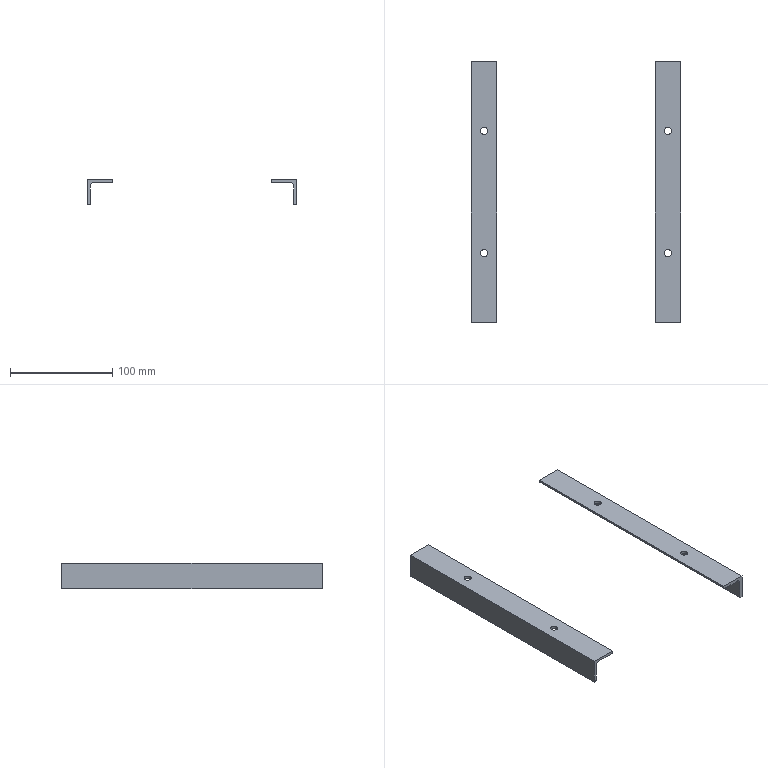Part | SolidWorks | features HoleWzd 1, WeldMemberFeat 1, WeldmentFeature 1 | 2 solids | 30 faces | box 205 x 255 x 25 mm | volume 72570 mm3 | plane 16 | cylinder 14 | commonest cylinder face diameters 7 x10 2 x4
STEP:
#1=CARTESIAN_POINT('',(-93.5,60.,-3.));
#2=VERTEX_POINT('',#1);
#3=CARTESIAN_POINT('',(-86.5,60.,-3.));
#4=VERTEX_POINT('',#3);
#5=CARTESIAN_POINT('',(-90.,60.,-3.));
#6=DIRECTION('',(0.,0.,1.));
#7=DIRECTION('',(1.,0.,0.));
#8=AXIS2_PLACEMENT_3D('',#5,#6,#7);
#9=CIRCLE('',#8,3.5);
#10=EDGE_CURVE('',#2,#4,#9,.T.);
#11=ORIENTED_EDGE('',*,*,#10,.F.);
#12=CARTESIAN_POINT('',(-93.5,60.,0.));
#13=VERTEX_POINT('',#12);
#14=CARTESIAN_POINT('',(-93.5,60.,0.));
#15=DIRECTION('',(0.,0.,1.));
#16=VECTOR('',#15,1000.);
#17=LINE('',#14,#16);
#18=EDGE_CURVE('',#2,#13,#17,.T.);
#19=ORIENTED_EDGE('',*,*,#18,.T.);
#20=CARTESIAN_POINT('',(-86.5,60.,0.));
#21=VERTEX_POINT('',#20);
#22=CARTESIAN_POINT('',(-90.,60.,0.));
#23=DIRECTION('',(0.,0.,1.));
#24=DIRECTION('',(1.,0.,0.));
#25=AXIS2_PLACEMENT_3D('',#22,#23,#24);
#26=CIRCLE('',#25,3.5);
#27=EDGE_CURVE('',#13,#21,#26,.T.);
#28=ORIENTED_EDGE('',*,*,#27,.T.);
#29=CARTESIAN_POINT('',(-86.5,60.,0.));
#30=DIRECTION('',(0.,0.,1.));
#31=VECTOR('',#30,1000.);
#32=LINE('',#29,#31);
#33=EDGE_CURVE('',#4,#21,#32,.T.);
#34=ORIENTED_EDGE('',*,*,#33,.F.);
#35=EDGE_LOOP('',(#11,#19,#28,#34));
#36=FACE_OUTER_BOUND('',#35,.T.);
#37=CARTESIAN_POINT('',(-90.,60.,0.));
#38=DIRECTION('',(0.,0.,1.));
#39=DIRECTION('',(1.,0.,0.));
#40=AXIS2_PLACEMENT_3D('',#37,#38,#39);
#41=CYLINDRICAL_SURFACE('',#40,3.5);
#42=ADVANCED_FACE('',(#36),#41,.F.);
#43=CARTESIAN_POINT('',(-93.5,-60.,-3.));
#44=VERTEX_POINT('',#43);
#45=CARTESIAN_POINT('',(-86.5,-60.,-3.));
#46=VERTEX_POINT('',#45);
#47=CARTESIAN_POINT('',(-90.,-60.,-3.));
#48=DIRECTION('',(0.,0.,1.));
#49=DIRECTION('',(1.,0.,0.));
#50=AXIS2_PLACEMENT_3D('',#47,#48,#49);
#51=CIRCLE('',#50,3.5);
#52=EDGE_CURVE('',#44,#46,#51,.T.);
#53=ORIENTED_EDGE('',*,*,#52,.F.);
#54=CARTESIAN_POINT('',(-93.5,-60.,0.));
#55=VERTEX_POINT('',#54);
#56=CARTESIAN_POINT('',(-93.5,-60.,0.));
#57=DIRECTION('',(0.,0.,1.));
#58=VECTOR('',#57,1000.);
#59=LINE('',#56,#58);
#60=EDGE_CURVE('',#44,#55,#59,.T.);
#61=ORIENTED_EDGE('',*,*,#60,.T.);
#62=CARTESIAN_POINT('',(-86.5,-60.,0.));
#63=VERTEX_POINT('',#62);
#64=CARTESIAN_POINT('',(-90.,-60.,0.));
#65=DIRECTION('',(0.,0.,1.));
#66=DIRECTION('',(1.,0.,0.));
#67=AXIS2_PLACEMENT_3D('',#64,#65,#66);
#68=CIRCLE('',#67,3.5);
#69=EDGE_CURVE('',#55,#63,#68,.T.);
#70=ORIENTED_EDGE('',*,*,#69,.T.);
#71=CARTESIAN_POINT('',(-86.5,-60.,0.));
#72=DIRECTION('',(0.,0.,1.));
#73=VECTOR('',#72,1000.);
#74=LINE('',#71,#73);
#75=EDGE_CURVE('',#46,#63,#74,.T.);
#76=ORIENTED_EDGE('',*,*,#75,.F.);
#77=EDGE_LOOP('',(#53,#61,#70,#76));
#78=FACE_OUTER_BOUND('',#77,.T.);
#79=CARTESIAN_POINT('',(-90.,-60.,0.));
#80=DIRECTION('',(0.,0.,1.));
#81=DIRECTION('',(1.,0.,0.));
#82=AXIS2_PLACEMENT_3D('',#79,#80,#81);
#83=CYLINDRICAL_SURFACE('',#82,3.5);
#84=ADVANCED_FACE('',(#78),#83,.F.);
#85=CARTESIAN_POINT('',(-100.5,-127.5,-25.));
#86=VERTEX_POINT('',#85);
#87=CARTESIAN_POINT('',(-102.5,-127.5,-25.));
#88=VERTEX_POINT('',#87);
#89=CARTESIAN_POINT('',(-102.5,-127.5,-25.));
#90=DIRECTION('',(-1.,0.,0.));
#91=VECTOR('',#90,1000.);
#92=LINE('',#89,#91);
#93=EDGE_CURVE('',#86,#88,#92,.T.);
#94=ORIENTED_EDGE('',*,*,#93,.T.);
#95=CARTESIAN_POINT('',(-102.5,127.5,-25.));
#96=VERTEX_POINT('',#95);
#97=CARTESIAN_POINT('',(-102.5,127.5,-25.));
#98=DIRECTION('',(0.,-1.,0.));
#99=VECTOR('',#98,1000.);
#100=LINE('',#97,#99);
#101=EDGE_CURVE('',#96,#88,#100,.T.);
#102=ORIENTED_EDGE('',*,*,#101,.F.);
#103=CARTESIAN_POINT('',(-100.5,127.5,-25.));
#104=VERTEX_POINT('',#103);
#105=CARTESIAN_POINT('',(-102.5,127.5,-25.));
#106=DIRECTION('',(-1.,0.,0.));
#107=VECTOR('',#106,1000.);
#108=LINE('',#105,#107);
#109=EDGE_CURVE('',#104,#96,#108,.T.);
#110=ORIENTED_EDGE('',*,*,#109,.F.);
#111=CARTESIAN_POINT('',(-100.5,127.5,-25.));
#112=DIRECTION('',(0.,-1.,0.));
#113=VECTOR('',#112,1000.);
#114=LINE('',#111,#113);
#115=EDGE_CURVE('',#104,#86,#114,.T.);
#116=ORIENTED_EDGE('',*,*,#115,.T.);
#117=EDGE_LOOP('',(#94,#102,#110,#116));
#118=FACE_OUTER_BOUND('',#117,.T.);
#119=CARTESIAN_POINT('',(-102.5,127.5,-25.));
#120=DIRECTION('',(0.,0.,1.));
#121=DIRECTION('',(1.,0.,0.));
#122=AXIS2_PLACEMENT_3D('',#119,#120,#121);
#123=PLANE('',#122);
#124=ADVANCED_FACE('',(#118),#123,.F.);
#125=CARTESIAN_POINT('',(-102.5,-127.5,0.));
#126=VERTEX_POINT('',#125);
#127=CARTESIAN_POINT('',(-102.5,-127.5,-25.));
#128=DIRECTION('',(0.,0.,1.));
#129=VECTOR('',#128,1000.);
#130=LINE('',#127,#129);
#131=EDGE_CURVE('',#88,#126,#130,.T.);
#132=ORIENTED_EDGE('',*,*,#131,.T.);
#133=CARTESIAN_POINT('',(-102.5,127.5,0.));
#134=VERTEX_POINT('',#133);
#135=CARTESIAN_POINT('',(-102.5,127.5,0.));
#136=DIRECTION('',(0.,-1.,0.));
#137=VECTOR('',#136,1000.);
#138=LINE('',#135,#137);
#139=EDGE_CURVE('',#134,#126,#138,.T.);
#140=ORIENTED_EDGE('',*,*,#139,.F.);
#141=CARTESIAN_POINT('',(-102.5,127.5,-25.));
#142=DIRECTION('',(0.,0.,1.));
#143=VECTOR('',#142,1000.);
#144=LINE('',#141,#143);
#145=EDGE_CURVE('',#96,#134,#144,.T.);
#146=ORIENTED_EDGE('',*,*,#145,.F.);
#147=ORIENTED_EDGE('',*,*,#101,.T.);
#148=EDGE_LOOP('',(#132,#140,#146,#147));
#149=FACE_OUTER_BOUND('',#148,.T.);
#150=CARTESIAN_POINT('',(-102.5,127.5,-25.));
#151=DIRECTION('',(1.,0.,0.));
#152=DIRECTION('',(0.,0.,-1.));
#153=AXIS2_PLACEMENT_3D('',#150,#151,#152);
#154=PLANE('',#153);
#155=ADVANCED_FACE('',(#149),#154,.F.);
#156=CARTESIAN_POINT('',(-90.,60.,0.));
#157=DIRECTION('',(0.,0.,1.));
#158=DIRECTION('',(1.,0.,0.));
#159=AXIS2_PLACEMENT_3D('',#156,#157,#158);
#160=CIRCLE('',#159,3.5);
#161=EDGE_CURVE('',#21,#13,#160,.T.);
#162=ORIENTED_EDGE('',*,*,#161,.F.);
#163=ORIENTED_EDGE('',*,*,#27,.F.);
#164=EDGE_LOOP('',(#162,#163));
#165=FACE_BOUND('',#164,.T.);
#166=CARTESIAN_POINT('',(-90.,-60.,0.));
#167=DIRECTION('',(0.,0.,1.));
#168=DIRECTION('',(1.,0.,0.));
#169=AXIS2_PLACEMENT_3D('',#166,#167,#168);
#170=CIRCLE('',#169,3.5);
#171=EDGE_CURVE('',#63,#55,#170,.T.);
#172=ORIENTED_EDGE('',*,*,#171,.F.);
#173=ORIENTED_EDGE('',*,*,#69,.F.);
#174=EDGE_LOOP('',(#172,#173));
#175=FACE_BOUND('',#174,.T.);
#176=CARTESIAN_POINT('',(-77.5,-127.5,0.));
#177=VERTEX_POINT('',#176);
#178=CARTESIAN_POINT('',(-102.5,-127.5,0.));
#179=DIRECTION('',(1.,0.,0.));
#180=VECTOR('',#179,1000.);
#181=LINE('',#178,#180);
#182=EDGE_CURVE('',#126,#177,#181,.T.);
#183=ORIENTED_EDGE('',*,*,#182,.T.);
#184=CARTESIAN_POINT('',(-77.5,127.5,0.));
#185=VERTEX_POINT('',#184);
#186=CARTESIAN_POINT('',(-77.5,127.5,0.));
#187=DIRECTION('',(0.,-1.,0.));
#188=VECTOR('',#187,1000.);
#189=LINE('',#186,#188);
#190=EDGE_CURVE('',#185,#177,#189,.T.);
#191=ORIENTED_EDGE('',*,*,#190,.F.);
#192=CARTESIAN_POINT('',(-102.5,127.5,0.));
#193=DIRECTION('',(1.,0.,0.));
#194=VECTOR('',#193,1000.);
#195=LINE('',#192,#194);
#196=EDGE_CURVE('',#134,#185,#195,.T.);
#197=ORIENTED_EDGE('',*,*,#196,.F.);
#198=ORIENTED_EDGE('',*,*,#139,.T.);
#199=EDGE_LOOP('',(#183,#191,#197,#198));
#200=FACE_OUTER_BOUND('',#199,.T.);
#201=CARTESIAN_POINT('',(-102.5,127.5,0.));
#202=DIRECTION('',(0.,0.,-1.));
#203=DIRECTION('',(-1.,0.,0.));
#204=AXIS2_PLACEMENT_3D('',#201,#202,#203);
#205=PLANE('',#204);
#206=ADVANCED_FACE('',(#165,#175,#200),#205,.F.);
#207=CARTESIAN_POINT('',(-77.5,-127.5,-2.));
#208=VERTEX_POINT('',#207);
#209=CARTESIAN_POINT('',(-77.5,-127.5,0.));
#210=DIRECTION('',(0.,0.,-1.));
#211=VECTOR('',#210,1000.);
#212=LINE('',#209,#211);
#213=EDGE_CURVE('',#177,#208,#212,.T.);
#214=ORIENTED_EDGE('',*,*,#213,.T.);
#215=CARTESIAN_POINT('',(-77.5,127.5,-2.));
#216=VERTEX_POINT('',#215);
#217=CARTESIAN_POINT('',(-77.5,127.5,-2.));
#218=DIRECTION('',(0.,-1.,0.));
#219=VECTOR('',#218,1000.);
#220=LINE('',#217,#219);
#221=EDGE_CURVE('',#216,#208,#220,.T.);
#222=ORIENTED_EDGE('',*,*,#221,.F.);
#223=CARTESIAN_POINT('',(-77.5,127.5,0.));
#224=DIRECTION('',(0.,0.,-1.));
#225=VECTOR('',#224,1000.);
#226=LINE('',#223,#225);
#227=EDGE_CURVE('',#185,#216,#226,.T.);
#228=ORIENTED_EDGE('',*,*,#227,.F.);
#229=ORIENTED_EDGE('',*,*,#190,.T.);
#230=EDGE_LOOP('',(#214,#222,#228,#229));
#231=FACE_OUTER_BOUND('',#230,.T.);
#232=CARTESIAN_POINT('',(-77.5,127.5,0.));
#233=DIRECTION('',(-1.,0.,0.));
#234=DIRECTION('',(0.,0.,1.));
#235=AXIS2_PLACEMENT_3D('',#232,#233,#234);
#236=PLANE('',#235);
#237=ADVANCED_FACE('',(#231),#236,.F.);
#238=CARTESIAN_POINT('',(-78.5,-127.5,-3.));
#239=VERTEX_POINT('',#238);
#240=CARTESIAN_POINT('',(-78.5,-127.5,-2.));
#241=DIRECTION('',(0.,1.,0.));
#242=DIRECTION('',(0.,0.,1.));
#243=AXIS2_PLACEMENT_3D('',#240,#241,#242);
#244=CIRCLE('',#243,1.);
#245=EDGE_CURVE('',#208,#239,#244,.T.);
#246=ORIENTED_EDGE('',*,*,#245,.T.);
#247=CARTESIAN_POINT('',(-78.5,127.5,-3.));
#248=VERTEX_POINT('',#247);
#249=CARTESIAN_POINT('',(-78.5,127.5,-3.));
#250=DIRECTION('',(0.,-1.,0.));
#251=VECTOR('',#250,1000.);
#252=LINE('',#249,#251);
#253=EDGE_CURVE('',#248,#239,#252,.T.);
#254=ORIENTED_EDGE('',*,*,#253,.F.);
#255=CARTESIAN_POINT('',(-78.5,127.5,-2.));
#256=DIRECTION('',(0.,1.,0.));
#257=DIRECTION('',(0.,0.,1.));
#258=AXIS2_PLACEMENT_3D('',#255,#256,#257);
#259=CIRCLE('',#258,1.);
#260=EDGE_CURVE('',#216,#248,#259,.T.);
#261=ORIENTED_EDGE('',*,*,#260,.F.);
#262=ORIENTED_EDGE('',*,*,#221,.T.);
#263=EDGE_LOOP('',(#246,#254,#261,#262));
#264=FACE_OUTER_BOUND('',#263,.T.);
#265=CARTESIAN_POINT('',(-78.5,127.5,-2.));
#266=DIRECTION('',(0.,-1.,0.));
#267=DIRECTION('',(0.,0.,-1.));
#268=AXIS2_PLACEMENT_3D('',#265,#266,#267);
#269=CYLINDRICAL_SURFACE('',#268,1.);
#270=ADVANCED_FACE('',(#264),#269,.T.);
#271=CARTESIAN_POINT('',(-90.,60.,-3.));
#272=DIRECTION('',(0.,0.,1.));
#273=DIRECTION('',(1.,0.,0.));
#274=AXIS2_PLACEMENT_3D('',#271,#272,#273);
#275=CIRCLE('',#274,3.5);
#276=EDGE_CURVE('',#4,#2,#275,.T.);
#277=ORIENTED_EDGE('',*,*,#276,.T.);
#278=ORIENTED_EDGE('',*,*,#10,.T.);
#279=EDGE_LOOP('',(#277,#278));
#280=FACE_BOUND('',#279,.T.);
#281=CARTESIAN_POINT('',(-90.,-60.,-3.));
#282=DIRECTION('',(0.,0.,1.));
#283=DIRECTION('',(1.,0.,0.));
#284=AXIS2_PLACEMENT_3D('',#281,#282,#283);
#285=CIRCLE('',#284,3.5);
#286=EDGE_CURVE('',#46,#44,#285,.T.);
#287=ORIENTED_EDGE('',*,*,#286,.T.);
#288=ORIENTED_EDGE('',*,*,#52,.T.);
#289=EDGE_LOOP('',(#287,#288));
#290=FACE_BOUND('',#289,.T.);
#291=CARTESIAN_POINT('',(-96.,-127.5,-3.));
#292=VERTEX_POINT('',#291);
#293=CARTESIAN_POINT('',(-96.,-127.5,-3.));
#294=DIRECTION('',(-1.,0.,0.));
#295=VECTOR('',#294,1000.);
#296=LINE('',#293,#295);
#297=EDGE_CURVE('',#239,#292,#296,.T.);
#298=ORIENTED_EDGE('',*,*,#297,.T.);
#299=CARTESIAN_POINT('',(-96.,127.5,-3.));
#300=VERTEX_POINT('',#299);
#301=CARTESIAN_POINT('',(-96.,127.5,-3.));
#302=DIRECTION('',(0.,-1.,0.));
#303=VECTOR('',#302,1000.);
#304=LINE('',#301,#303);
#305=EDGE_CURVE('',#300,#292,#304,.T.);
#306=ORIENTED_EDGE('',*,*,#305,.F.);
#307=CARTESIAN_POINT('',(-96.,127.5,-3.));
#308=DIRECTION('',(-1.,0.,0.));
#309=VECTOR('',#308,1000.);
#310=LINE('',#307,#309);
#311=EDGE_CURVE('',#248,#300,#310,.T.);
#312=ORIENTED_EDGE('',*,*,#311,.F.);
#313=ORIENTED_EDGE('',*,*,#253,.T.);
#314=EDGE_LOOP('',(#298,#306,#312,#313));
#315=FACE_OUTER_BOUND('',#314,.T.);
#316=CARTESIAN_POINT('',(-96.,127.5,-3.));
#317=DIRECTION('',(0.,0.,1.));
#318=DIRECTION('',(1.,0.,0.));
#319=AXIS2_PLACEMENT_3D('',#316,#317,#318);
#320=PLANE('',#319);
#321=ADVANCED_FACE('',(#280,#290,#315),#320,.F.);
#322=CARTESIAN_POINT('',(-99.5,-127.5,-6.5));
#323=VERTEX_POINT('',#322);
#324=CARTESIAN_POINT('',(-96.,-127.5,-6.5));
#325=DIRECTION('',(0.,-1.,0.));
#326=DIRECTION('',(0.,0.,1.));
#327=AXIS2_PLACEMENT_3D('',#324,#325,#326);
#328=CIRCLE('',#327,3.5);
#329=EDGE_CURVE('',#292,#323,#328,.T.);
#330=ORIENTED_EDGE('',*,*,#329,.T.);
#331=CARTESIAN_POINT('',(-99.5,127.5,-6.5));
#332=VERTEX_POINT('',#331);
#333=CARTESIAN_POINT('',(-99.5,127.5,-6.5));
#334=DIRECTION('',(0.,-1.,0.));
#335=VECTOR('',#334,1000.);
#336=LINE('',#333,#335);
#337=EDGE_CURVE('',#332,#323,#336,.T.);
#338=ORIENTED_EDGE('',*,*,#337,.F.);
#339=CARTESIAN_POINT('',(-96.,127.5,-6.5));
#340=DIRECTION('',(0.,-1.,0.));
#341=DIRECTION('',(0.,0.,1.));
#342=AXIS2_PLACEMENT_3D('',#339,#340,#341);
#343=CIRCLE('',#342,3.5);
#344=EDGE_CURVE('',#300,#332,#343,.T.);
#345=ORIENTED_EDGE('',*,*,#344,.F.);
#346=ORIENTED_EDGE('',*,*,#305,.T.);
#347=EDGE_LOOP('',(#330,#338,#345,#346));
#348=FACE_OUTER_BOUND('',#347,.T.);
#349=CARTESIAN_POINT('',(-96.,127.5,-6.5));
#350=DIRECTION('',(0.,-1.,0.));
#351=DIRECTION('',(0.,0.,-1.));
#352=AXIS2_PLACEMENT_3D('',#349,#350,#351);
#353=CYLINDRICAL_SURFACE('',#352,3.5);
#354=ADVANCED_FACE('',(#348),#353,.F.);
#355=CARTESIAN_POINT('',(-99.5,-127.5,-24.));
#356=VERTEX_POINT('',#355);
#357=CARTESIAN_POINT('',(-99.5,-127.5,-24.));
#358=DIRECTION('',(0.,0.,-1.));
#359=VECTOR('',#358,1000.);
#360=LINE('',#357,#359);
#361=EDGE_CURVE('',#323,#356,#360,.T.);
#362=ORIENTED_EDGE('',*,*,#361,.T.);
#363=CARTESIAN_POINT('',(-99.5,127.5,-24.));
#364=VERTEX_POINT('',#363);
#365=CARTESIAN_POINT('',(-99.5,127.5,-24.));
#366=DIRECTION('',(0.,-1.,0.));
#367=VECTOR('',#366,1000.);
#368=LINE('',#365,#367);
#369=EDGE_CURVE('',#364,#356,#368,.T.);
#370=ORIENTED_EDGE('',*,*,#369,.F.);
#371=CARTESIAN_POINT('',(-99.5,127.5,-24.));
#372=DIRECTION('',(0.,0.,-1.));
#373=VECTOR('',#372,1000.);
#374=LINE('',#371,#373);
#375=EDGE_CURVE('',#332,#364,#374,.T.);
#376=ORIENTED_EDGE('',*,*,#375,.F.);
#377=ORIENTED_EDGE('',*,*,#337,.T.);
#378=EDGE_LOOP('',(#362,#370,#376,#377));
#379=FACE_OUTER_BOUND('',#378,.T.);
#380=CARTESIAN_POINT('',(-99.5,127.5,-24.));
#381=DIRECTION('',(-1.,0.,0.));
#382=DIRECTION('',(0.,0.,1.));
#383=AXIS2_PLACEMENT_3D('',#380,#381,#382);
#384=PLANE('',#383);
#385=ADVANCED_FACE('',(#379),#384,.F.);
#386=CARTESIAN_POINT('',(-100.5,-127.5,-24.));
#387=DIRECTION('',(0.,1.,0.));
#388=DIRECTION('',(0.,0.,-1.));
#389=AXIS2_PLACEMENT_3D('',#386,#387,#388);
#390=CIRCLE('',#389,1.);
#391=EDGE_CURVE('',#356,#86,#390,.T.);
#392=ORIENTED_EDGE('',*,*,#391,.T.);
#393=ORIENTED_EDGE('',*,*,#115,.F.);
#394=CARTESIAN_POINT('',(-100.5,127.5,-24.));
#395=DIRECTION('',(0.,1.,0.));
#396=DIRECTION('',(0.,0.,-1.));
#397=AXIS2_PLACEMENT_3D('',#394,#395,#396);
#398=CIRCLE('',#397,1.);
#399=EDGE_CURVE('',#364,#104,#398,.T.);
#400=ORIENTED_EDGE('',*,*,#399,.F.);
#401=ORIENTED_EDGE('',*,*,#369,.T.);
#402=EDGE_LOOP('',(#392,#393,#400,#401));
#403=FACE_OUTER_BOUND('',#402,.T.);
#404=CARTESIAN_POINT('',(-100.5,127.5,-24.));
#405=DIRECTION('',(0.,-1.,0.));
#406=DIRECTION('',(0.,0.,-1.));
#407=AXIS2_PLACEMENT_3D('',#404,#405,#406);
#408=CYLINDRICAL_SURFACE('',#407,1.);
#409=ADVANCED_FACE('',(#403),#408,.T.);
#410=ORIENTED_EDGE('',*,*,#109,.T.);
#411=ORIENTED_EDGE('',*,*,#145,.T.);
#412=ORIENTED_EDGE('',*,*,#196,.T.);
#413=ORIENTED_EDGE('',*,*,#227,.T.);
#414=ORIENTED_EDGE('',*,*,#260,.T.);
#415=ORIENTED_EDGE('',*,*,#311,.T.);
#416=ORIENTED_EDGE('',*,*,#344,.T.);
#417=ORIENTED_EDGE('',*,*,#375,.T.);
#418=ORIENTED_EDGE('',*,*,#399,.T.);
#419=EDGE_LOOP('',(#410,#411,#412,#413,#414,#415,#416,#417,#418));
#420=FACE_OUTER_BOUND('',#419,.T.);
#421=CARTESIAN_POINT('',(-100.5,127.5,-24.));
#422=DIRECTION('',(0.,-1.,0.));
#423=DIRECTION('',(0.,0.,-1.));
#424=AXIS2_PLACEMENT_3D('',#421,#422,#423);
#425=PLANE('',#424);
#426=ADVANCED_FACE('',(#420),#425,.F.);
#427=ORIENTED_EDGE('',*,*,#93,.F.);
#428=ORIENTED_EDGE('',*,*,#391,.F.);
#429=ORIENTED_EDGE('',*,*,#361,.F.);
#430=ORIENTED_EDGE('',*,*,#329,.F.);
#431=ORIENTED_EDGE('',*,*,#297,.F.);
#432=ORIENTED_EDGE('',*,*,#245,.F.);
#433=ORIENTED_EDGE('',*,*,#213,.F.);
#434=ORIENTED_EDGE('',*,*,#182,.F.);
#435=ORIENTED_EDGE('',*,*,#131,.F.);
#436=EDGE_LOOP('',(#427,#428,#429,#430,#431,#432,#433,#434,#435));
#437=FACE_OUTER_BOUND('',#436,.T.);
#438=CARTESIAN_POINT('',(-100.5,-127.5,-24.));
#439=DIRECTION('',(0.,-1.,0.));
#440=DIRECTION('',(0.,0.,-1.));
#441=AXIS2_PLACEMENT_3D('',#438,#439,#440);
#442=PLANE('',#441);
#443=ADVANCED_FACE('',(#437),#442,.T.);
#444=ORIENTED_EDGE('',*,*,#60,.F.);
#445=ORIENTED_EDGE('',*,*,#286,.F.);
#446=ORIENTED_EDGE('',*,*,#75,.T.);
#447=ORIENTED_EDGE('',*,*,#171,.T.);
#448=EDGE_LOOP('',(#444,#445,#446,#447));
#449=FACE_OUTER_BOUND('',#448,.T.);
#450=CARTESIAN_POINT('',(-90.,-60.,0.));
#451=DIRECTION('',(0.,0.,1.));
#452=DIRECTION('',(1.,0.,0.));
#453=AXIS2_PLACEMENT_3D('',#450,#451,#452);
#454=CYLINDRICAL_SURFACE('',#453,3.5);
#455=ADVANCED_FACE('',(#449),#454,.F.);
#456=ORIENTED_EDGE('',*,*,#18,.F.);
#457=ORIENTED_EDGE('',*,*,#276,.F.);
#458=ORIENTED_EDGE('',*,*,#33,.T.);
#459=ORIENTED_EDGE('',*,*,#161,.T.);
#460=EDGE_LOOP('',(#456,#457,#458,#459));
#461=FACE_OUTER_BOUND('',#460,.T.);
#462=CARTESIAN_POINT('',(-90.,60.,0.));
#463=DIRECTION('',(0.,0.,1.));
#464=DIRECTION('',(1.,0.,0.));
#465=AXIS2_PLACEMENT_3D('',#462,#463,#464);
#466=CYLINDRICAL_SURFACE('',#465,3.5);
#467=ADVANCED_FACE('',(#461),#466,.F.);
#468=CLOSED_SHELL('',(#42,#84,#124,#155,#206,#237,#270,#321,#354,#385,#409,#426,#443,#455,#467));
#469=MANIFOLD_SOLID_BREP('',#468);
#470=CARTESIAN_POINT('',(93.5,-60.,-3.));
#471=VERTEX_POINT('',#470);
#472=CARTESIAN_POINT('',(86.5,-60.,-3.));
#473=VERTEX_POINT('',#472);
#474=CARTESIAN_POINT('',(90.,-60.,-3.));
#475=DIRECTION('',(0.,0.,-1.));
#476=DIRECTION('',(-1.,0.,0.));
#477=AXIS2_PLACEMENT_3D('',#474,#475,#476);
#478=CIRCLE('',#477,3.5);
#479=EDGE_CURVE('',#471,#473,#478,.T.);
#480=ORIENTED_EDGE('',*,*,#479,.T.);
#481=CARTESIAN_POINT('',(86.5,-60.,0.));
#482=VERTEX_POINT('',#481);
#483=CARTESIAN_POINT('',(86.5,-60.,0.));
#484=DIRECTION('',(0.,0.,1.));
#485=VECTOR('',#484,1000.);
#486=LINE('',#483,#485);
#487=EDGE_CURVE('',#473,#482,#486,.T.);
#488=ORIENTED_EDGE('',*,*,#487,.T.);
#489=CARTESIAN_POINT('',(93.5,-60.,0.));
#490=VERTEX_POINT('',#489);
#491=CARTESIAN_POINT('',(90.,-60.,0.));
#492=DIRECTION('',(0.,0.,1.));
#493=DIRECTION('',(1.,0.,0.));
#494=AXIS2_PLACEMENT_3D('',#491,#492,#493);
#495=CIRCLE('',#494,3.5);
#496=EDGE_CURVE('',#482,#490,#495,.T.);
#497=ORIENTED_EDGE('',*,*,#496,.T.);
#498=CARTESIAN_POINT('',(93.5,-60.,0.));
#499=DIRECTION('',(0.,0.,1.));
#500=VECTOR('',#499,1000.);
#501=LINE('',#498,#500);
#502=EDGE_CURVE('',#471,#490,#501,.T.);
#503=ORIENTED_EDGE('',*,*,#502,.F.);
#504=EDGE_LOOP('',(#480,#488,#497,#503));
#505=FACE_OUTER_BOUND('',#504,.T.);
#506=CARTESIAN_POINT('',(90.,-60.,0.));
#507=DIRECTION('',(0.,0.,1.));
#508=DIRECTION('',(1.,0.,0.));
#509=AXIS2_PLACEMENT_3D('',#506,#507,#508);
#510=CYLINDRICAL_SURFACE('',#509,3.5);
#511=ADVANCED_FACE('',(#505),#510,.F.);
#512=CARTESIAN_POINT('',(93.5,60.,-3.));
#513=VERTEX_POINT('',#512);
#514=CARTESIAN_POINT('',(86.5,60.,-3.));
#515=VERTEX_POINT('',#514);
#516=CARTESIAN_POINT('',(90.,60.,-3.));
#517=DIRECTION('',(0.,0.,-1.));
#518=DIRECTION('',(-1.,0.,0.));
#519=AXIS2_PLACEMENT_3D('',#516,#517,#518);
#520=CIRCLE('',#519,3.5);
#521=EDGE_CURVE('',#513,#515,#520,.T.);
#522=ORIENTED_EDGE('',*,*,#521,.T.);
#523=CARTESIAN_POINT('',(86.5,60.,0.));
#524=VERTEX_POINT('',#523);
#525=CARTESIAN_POINT('',(86.5,60.,0.));
#526=DIRECTION('',(0.,0.,1.));
#527=VECTOR('',#526,1000.);
#528=LINE('',#525,#527);
#529=EDGE_CURVE('',#515,#524,#528,.T.);
#530=ORIENTED_EDGE('',*,*,#529,.T.);
#531=CARTESIAN_POINT('',(93.5,60.,0.));
#532=VERTEX_POINT('',#531);
#533=CARTESIAN_POINT('',(90.,60.,0.));
#534=DIRECTION('',(0.,0.,1.));
#535=DIRECTION('',(1.,0.,0.));
#536=AXIS2_PLACEMENT_3D('',#533,#534,#535);
#537=CIRCLE('',#536,3.5);
#538=EDGE_CURVE('',#524,#532,#537,.T.);
#539=ORIENTED_EDGE('',*,*,#538,.T.);
#540=CARTESIAN_POINT('',(93.5,60.,0.));
#541=DIRECTION('',(0.,0.,1.));
#542=VECTOR('',#541,1000.);
#543=LINE('',#540,#542);
#544=EDGE_CURVE('',#513,#532,#543,.T.);
#545=ORIENTED_EDGE('',*,*,#544,.F.);
#546=EDGE_LOOP('',(#522,#530,#539,#545));
#547=FACE_OUTER_BOUND('',#546,.T.);
#548=CARTESIAN_POINT('',(90.,60.,0.));
#549=DIRECTION('',(0.,0.,1.));
#550=DIRECTION('',(1.,0.,0.));
#551=AXIS2_PLACEMENT_3D('',#548,#549,#550);
#552=CYLINDRICAL_SURFACE('',#551,3.5);
#553=ADVANCED_FACE('',(#547),#552,.F.);
#554=CARTESIAN_POINT('',(77.5,127.5,-2.));
#555=VERTEX_POINT('',#554);
#556=CARTESIAN_POINT('',(77.5,127.5,0.));
#557=VERTEX_POINT('',#556);
#558=CARTESIAN_POINT('',(77.5,127.5,0.));
#559=DIRECTION('',(0.,0.,1.));
#560=VECTOR('',#559,1000.);
#561=LINE('',#558,#560);
#562=EDGE_CURVE('',#555,#557,#561,.T.);
#563=ORIENTED_EDGE('',*,*,#562,.F.);
#564=CARTESIAN_POINT('',(77.5,-127.5,-2.));
#565=VERTEX_POINT('',#564);
#566=CARTESIAN_POINT('',(77.5,-127.5,-2.));
#567=DIRECTION('',(0.,1.,0.));
#568=VECTOR('',#567,1000.);
#569=LINE('',#566,#568);
#570=EDGE_CURVE('',#565,#555,#569,.T.);
#571=ORIENTED_EDGE('',*,*,#570,.F.);
#572=CARTESIAN_POINT('',(77.5,-127.5,0.));
#573=VERTEX_POINT('',#572);
#574=CARTESIAN_POINT('',(77.5,-127.5,0.));
#575=DIRECTION('',(0.,0.,1.));
#576=VECTOR('',#575,1000.);
#577=LINE('',#574,#576);
#578=EDGE_CURVE('',#565,#573,#577,.T.);
#579=ORIENTED_EDGE('',*,*,#578,.T.);
#580=CARTESIAN_POINT('',(77.5,-127.5,0.));
#581=DIRECTION('',(0.,1.,0.));
#582=VECTOR('',#581,1000.);
#583=LINE('',#580,#582);
#584=EDGE_CURVE('',#573,#557,#583,.T.);
#585=ORIENTED_EDGE('',*,*,#584,.T.);
#586=EDGE_LOOP('',(#563,#571,#579,#585));
#587=FACE_OUTER_BOUND('',#586,.T.);
#588=CARTESIAN_POINT('',(77.5,-127.5,0.));
#589=DIRECTION('',(-1.,0.,0.));
#590=DIRECTION('',(0.,0.,1.));
#591=AXIS2_PLACEMENT_3D('',#588,#589,#590);
#592=PLANE('',#591);
#593=ADVANCED_FACE('',(#587),#592,.T.);
#594=CARTESIAN_POINT('',(78.5,127.5,-3.));
#595=VERTEX_POINT('',#594);
#596=CARTESIAN_POINT('',(78.5,127.5,-2.));
#597=DIRECTION('',(0.,1.,0.));
#598=DIRECTION('',(-1.,0.,0.));
#599=AXIS2_PLACEMENT_3D('',#596,#597,#598);
#600=CIRCLE('',#599,1.);
#601=EDGE_CURVE('',#595,#555,#600,.T.);
#602=ORIENTED_EDGE('',*,*,#601,.F.);
#603=CARTESIAN_POINT('',(78.5,-127.5,-3.));
#604=VERTEX_POINT('',#603);
#605=CARTESIAN_POINT('',(78.5,-127.5,-3.));
#606=DIRECTION('',(0.,1.,0.));
#607=VECTOR('',#606,1000.);
#608=LINE('',#605,#607);
#609=EDGE_CURVE('',#604,#595,#608,.T.);
#610=ORIENTED_EDGE('',*,*,#609,.F.);
#611=CARTESIAN_POINT('',(78.5,-127.5,-2.));
#612=DIRECTION('',(0.,1.,0.));
#613=DIRECTION('',(-1.,0.,0.));
#614=AXIS2_PLACEMENT_3D('',#611,#612,#613);
#615=CIRCLE('',#614,1.);
#616=EDGE_CURVE('',#604,#565,#615,.T.);
#617=ORIENTED_EDGE('',*,*,#616,.T.);
#618=ORIENTED_EDGE('',*,*,#570,.T.);
#619=EDGE_LOOP('',(#602,#610,#617,#618));
#620=FACE_OUTER_BOUND('',#619,.T.);
#621=CARTESIAN_POINT('',(78.5,-127.5,-2.));
#622=DIRECTION('',(0.,1.,0.));
#623=DIRECTION('',(0.,0.,1.));
#624=AXIS2_PLACEMENT_3D('',#621,#622,#623);
#625=CYLINDRICAL_SURFACE('',#624,1.);
#626=ADVANCED_FACE('',(#620),#625,.T.);
#627=ORIENTED_EDGE('',*,*,#479,.F.);
#628=CARTESIAN_POINT('',(90.,-60.,-3.));
#629=DIRECTION('',(0.,0.,-1.));
#630=DIRECTION('',(-1.,0.,0.));
#631=AXIS2_PLACEMENT_3D('',#628,#629,#630);
#632=CIRCLE('',#631,3.5);
#633=EDGE_CURVE('',#473,#471,#632,.T.);
#634=ORIENTED_EDGE('',*,*,#633,.F.);
#635=EDGE_LOOP('',(#627,#634));
#636=FACE_BOUND('',#635,.T.);
#637=ORIENTED_EDGE('',*,*,#521,.F.);
#638=CARTESIAN_POINT('',(90.,60.,-3.));
#639=DIRECTION('',(0.,0.,-1.));
#640=DIRECTION('',(-1.,0.,0.));
#641=AXIS2_PLACEMENT_3D('',#638,#639,#640);
#642=CIRCLE('',#641,3.5);
#643=EDGE_CURVE('',#515,#513,#642,.T.);
#644=ORIENTED_EDGE('',*,*,#643,.F.);
#645=EDGE_LOOP('',(#637,#644));
#646=FACE_BOUND('',#645,.T.);
#647=CARTESIAN_POINT('',(96.,127.5,-3.));
#648=VERTEX_POINT('',#647);
#649=CARTESIAN_POINT('',(78.5,127.5,-3.));
#650=DIRECTION('',(-1.,0.,0.));
#651=VECTOR('',#650,1000.);
#652=LINE('',#649,#651);
#653=EDGE_CURVE('',#648,#595,#652,.T.);
#654=ORIENTED_EDGE('',*,*,#653,.F.);
#655=CARTESIAN_POINT('',(96.,-127.5,-3.));
#656=VERTEX_POINT('',#655);
#657=CARTESIAN_POINT('',(96.,-127.5,-3.));
#658=DIRECTION('',(0.,1.,0.));
#659=VECTOR('',#658,1000.);
#660=LINE('',#657,#659);
#661=EDGE_CURVE('',#656,#648,#660,.T.);
#662=ORIENTED_EDGE('',*,*,#661,.F.);
#663=CARTESIAN_POINT('',(78.5,-127.5,-3.));
#664=DIRECTION('',(-1.,0.,0.));
#665=VECTOR('',#664,1000.);
#666=LINE('',#663,#665);
#667=EDGE_CURVE('',#656,#604,#666,.T.);
#668=ORIENTED_EDGE('',*,*,#667,.T.);
#669=ORIENTED_EDGE('',*,*,#609,.T.);
#670=EDGE_LOOP('',(#654,#662,#668,#669));
#671=FACE_OUTER_BOUND('',#670,.T.);
#672=CARTESIAN_POINT('',(78.5,-127.5,-3.));
#673=DIRECTION('',(0.,0.,-1.));
#674=DIRECTION('',(-1.,0.,0.));
#675=AXIS2_PLACEMENT_3D('',#672,#673,#674);
#676=PLANE('',#675);
#677=ADVANCED_FACE('',(#636,#646,#671),#676,.T.);
#678=CARTESIAN_POINT('',(99.5,127.5,-6.5));
#679=VERTEX_POINT('',#678);
#680=CARTESIAN_POINT('',(96.,127.5,-6.5));
#681=DIRECTION('',(0.,-1.,0.));
#682=DIRECTION('',(1.,0.,0.));
#683=AXIS2_PLACEMENT_3D('',#680,#681,#682);
#684=CIRCLE('',#683,3.5);
#685=EDGE_CURVE('',#679,#648,#684,.T.);
#686=ORIENTED_EDGE('',*,*,#685,.F.);
#687=CARTESIAN_POINT('',(99.5,-127.5,-6.5));
#688=VERTEX_POINT('',#687);
#689=CARTESIAN_POINT('',(99.5,-127.5,-6.5));
#690=DIRECTION('',(0.,1.,0.));
#691=VECTOR('',#690,1000.);
#692=LINE('',#689,#691);
#693=EDGE_CURVE('',#688,#679,#692,.T.);
#694=ORIENTED_EDGE('',*,*,#693,.F.);
#695=CARTESIAN_POINT('',(96.,-127.5,-6.5));
#696=DIRECTION('',(0.,-1.,0.));
#697=DIRECTION('',(1.,0.,0.));
#698=AXIS2_PLACEMENT_3D('',#695,#696,#697);
#699=CIRCLE('',#698,3.5);
#700=EDGE_CURVE('',#688,#656,#699,.T.);
#701=ORIENTED_EDGE('',*,*,#700,.T.);
#702=ORIENTED_EDGE('',*,*,#661,.T.);
#703=EDGE_LOOP('',(#686,#694,#701,#702));
#704=FACE_OUTER_BOUND('',#703,.T.);
#705=CARTESIAN_POINT('',(96.,-127.5,-6.5));
#706=DIRECTION('',(0.,1.,0.));
#707=DIRECTION('',(0.,0.,1.));
#708=AXIS2_PLACEMENT_3D('',#705,#706,#707);
#709=CYLINDRICAL_SURFACE('',#708,3.5);
#710=ADVANCED_FACE('',(#704),#709,.F.);
#711=CARTESIAN_POINT('',(99.5,127.5,-24.));
#712=VERTEX_POINT('',#711);
#713=CARTESIAN_POINT('',(99.5,127.5,-6.5));
#714=DIRECTION('',(0.,0.,1.));
#715=VECTOR('',#714,1000.);
#716=LINE('',#713,#715);
#717=EDGE_CURVE('',#712,#679,#716,.T.);
#718=ORIENTED_EDGE('',*,*,#717,.F.);
#719=CARTESIAN_POINT('',(99.5,-127.5,-24.));
#720=VERTEX_POINT('',#719);
#721=CARTESIAN_POINT('',(99.5,-127.5,-24.));
#722=DIRECTION('',(0.,1.,0.));
#723=VECTOR('',#722,1000.);
#724=LINE('',#721,#723);
#725=EDGE_CURVE('',#720,#712,#724,.T.);
#726=ORIENTED_EDGE('',*,*,#725,.F.);
#727=CARTESIAN_POINT('',(99.5,-127.5,-6.5));
#728=DIRECTION('',(0.,0.,1.));
#729=VECTOR('',#728,1000.);
#730=LINE('',#727,#729);
#731=EDGE_CURVE('',#720,#688,#730,.T.);
#732=ORIENTED_EDGE('',*,*,#731,.T.);
#733=ORIENTED_EDGE('',*,*,#693,.T.);
#734=EDGE_LOOP('',(#718,#726,#732,#733));
#735=FACE_OUTER_BOUND('',#734,.T.);
#736=CARTESIAN_POINT('',(99.5,-127.5,-6.5));
#737=DIRECTION('',(-1.,0.,0.));
#738=DIRECTION('',(0.,0.,1.));
#739=AXIS2_PLACEMENT_3D('',#736,#737,#738);
#740=PLANE('',#739);
#741=ADVANCED_FACE('',(#735),#740,.T.);
#742=CARTESIAN_POINT('',(100.5,127.5,-25.));
#743=VERTEX_POINT('',#742);
#744=CARTESIAN_POINT('',(100.5,127.5,-24.));
#745=DIRECTION('',(0.,1.,0.));
#746=DIRECTION('',(1.,0.,0.));
#747=AXIS2_PLACEMENT_3D('',#744,#745,#746);
#748=CIRCLE('',#747,1.);
#749=EDGE_CURVE('',#743,#712,#748,.T.);
#750=ORIENTED_EDGE('',*,*,#749,.F.);
#751=CARTESIAN_POINT('',(100.5,-127.5,-25.));
#752=VERTEX_POINT('',#751);
#753=CARTESIAN_POINT('',(100.5,-127.5,-25.));
#754=DIRECTION('',(0.,1.,0.));
#755=VECTOR('',#754,1000.);
#756=LINE('',#753,#755);
#757=EDGE_CURVE('',#752,#743,#756,.T.);
#758=ORIENTED_EDGE('',*,*,#757,.F.);
#759=CARTESIAN_POINT('',(100.5,-127.5,-24.));
#760=DIRECTION('',(0.,1.,0.));
#761=DIRECTION('',(1.,0.,0.));
#762=AXIS2_PLACEMENT_3D('',#759,#760,#761);
#763=CIRCLE('',#762,1.);
#764=EDGE_CURVE('',#752,#720,#763,.T.);
#765=ORIENTED_EDGE('',*,*,#764,.T.);
#766=ORIENTED_EDGE('',*,*,#725,.T.);
#767=EDGE_LOOP('',(#750,#758,#765,#766));
#768=FACE_OUTER_BOUND('',#767,.T.);
#769=CARTESIAN_POINT('',(100.5,-127.5,-24.));
#770=DIRECTION('',(0.,1.,0.));
#771=DIRECTION('',(0.,0.,1.));
#772=AXIS2_PLACEMENT_3D('',#769,#770,#771);
#773=CYLINDRICAL_SURFACE('',#772,1.);
#774=ADVANCED_FACE('',(#768),#773,.T.);
#775=CARTESIAN_POINT('',(102.5,127.5,-25.));
#776=VERTEX_POINT('',#775);
#777=CARTESIAN_POINT('',(102.5,127.5,-25.));
#778=DIRECTION('',(-1.,0.,0.));
#779=VECTOR('',#778,1000.);
#780=LINE('',#777,#779);
#781=EDGE_CURVE('',#776,#743,#780,.T.);
#782=ORIENTED_EDGE('',*,*,#781,.F.);
#783=CARTESIAN_POINT('',(102.5,-127.5,-25.));
#784=VERTEX_POINT('',#783);
#785=CARTESIAN_POINT('',(102.5,-127.5,-25.));
#786=DIRECTION('',(0.,1.,0.));
#787=VECTOR('',#786,1000.);
#788=LINE('',#785,#787);
#789=EDGE_CURVE('',#784,#776,#788,.T.);
#790=ORIENTED_EDGE('',*,*,#789,.F.);
#791=CARTESIAN_POINT('',(102.5,-127.5,-25.));
#792=DIRECTION('',(-1.,0.,0.));
#793=VECTOR('',#792,1000.);
#794=LINE('',#791,#793);
#795=EDGE_CURVE('',#784,#752,#794,.T.);
#796=ORIENTED_EDGE('',*,*,#795,.T.);
#797=ORIENTED_EDGE('',*,*,#757,.T.);
#798=EDGE_LOOP('',(#782,#790,#796,#797));
#799=FACE_OUTER_BOUND('',#798,.T.);
#800=CARTESIAN_POINT('',(102.5,-127.5,-25.));
#801=DIRECTION('',(0.,0.,-1.));
#802=DIRECTION('',(-1.,0.,0.));
#803=AXIS2_PLACEMENT_3D('',#800,#801,#802);
#804=PLANE('',#803);
#805=ADVANCED_FACE('',(#799),#804,.T.);
#806=CARTESIAN_POINT('',(102.5,127.5,0.));
#807=VERTEX_POINT('',#806);
#808=CARTESIAN_POINT('',(102.5,127.5,0.));
#809=DIRECTION('',(0.,0.,-1.));
#810=VECTOR('',#809,1000.);
#811=LINE('',#808,#810);
#812=EDGE_CURVE('',#807,#776,#811,.T.);
#813=ORIENTED_EDGE('',*,*,#812,.F.);
#814=CARTESIAN_POINT('',(102.5,-127.5,0.));
#815=VERTEX_POINT('',#814);
#816=CARTESIAN_POINT('',(102.5,-127.5,0.));
#817=DIRECTION('',(0.,1.,0.));
#818=VECTOR('',#817,1000.);
#819=LINE('',#816,#818);
#820=EDGE_CURVE('',#815,#807,#819,.T.);
#821=ORIENTED_EDGE('',*,*,#820,.F.);
#822=CARTESIAN_POINT('',(102.5,-127.5,0.));
#823=DIRECTION('',(0.,0.,-1.));
#824=VECTOR('',#823,1000.);
#825=LINE('',#822,#824);
#826=EDGE_CURVE('',#815,#784,#825,.T.);
#827=ORIENTED_EDGE('',*,*,#826,.T.);
#828=ORIENTED_EDGE('',*,*,#789,.T.);
#829=EDGE_LOOP('',(#813,#821,#827,#828));
#830=FACE_OUTER_BOUND('',#829,.T.);
#831=CARTESIAN_POINT('',(102.5,-127.5,0.));
#832=DIRECTION('',(1.,0.,0.));
#833=DIRECTION('',(0.,0.,-1.));
#834=AXIS2_PLACEMENT_3D('',#831,#832,#833);
#835=PLANE('',#834);
#836=ADVANCED_FACE('',(#830),#835,.T.);
#837=CARTESIAN_POINT('',(90.,-60.,0.));
#838=DIRECTION('',(0.,0.,1.));
#839=DIRECTION('',(1.,0.,0.));
#840=AXIS2_PLACEMENT_3D('',#837,#838,#839);
#841=CIRCLE('',#840,3.5);
#842=EDGE_CURVE('',#490,#482,#841,.T.);
#843=ORIENTED_EDGE('',*,*,#842,.F.);
#844=ORIENTED_EDGE('',*,*,#496,.F.);
#845=EDGE_LOOP('',(#843,#844));
#846=FACE_BOUND('',#845,.T.);
#847=CARTESIAN_POINT('',(90.,60.,0.));
#848=DIRECTION('',(0.,0.,1.));
#849=DIRECTION('',(1.,0.,0.));
#850=AXIS2_PLACEMENT_3D('',#847,#848,#849);
#851=CIRCLE('',#850,3.5);
#852=EDGE_CURVE('',#532,#524,#851,.T.);
#853=ORIENTED_EDGE('',*,*,#852,.F.);
#854=ORIENTED_EDGE('',*,*,#538,.F.);
#855=EDGE_LOOP('',(#853,#854));
#856=FACE_BOUND('',#855,.T.);
#857=CARTESIAN_POINT('',(77.5,127.5,0.));
#858=DIRECTION('',(1.,0.,0.));
#859=VECTOR('',#858,1000.);
#860=LINE('',#857,#859);
#861=EDGE_CURVE('',#557,#807,#860,.T.);
#862=ORIENTED_EDGE('',*,*,#861,.F.);
#863=ORIENTED_EDGE('',*,*,#584,.F.);
#864=CARTESIAN_POINT('',(77.5,-127.5,0.));
#865=DIRECTION('',(1.,0.,0.));
#866=VECTOR('',#865,1000.);
#867=LINE('',#864,#866);
#868=EDGE_CURVE('',#573,#815,#867,.T.);
#869=ORIENTED_EDGE('',*,*,#868,.T.);
#870=ORIENTED_EDGE('',*,*,#820,.T.);
#871=EDGE_LOOP('',(#862,#863,#869,#870));
#872=FACE_OUTER_BOUND('',#871,.T.);
#873=CARTESIAN_POINT('',(77.5,-127.5,0.));
#874=DIRECTION('',(0.,0.,1.));
#875=DIRECTION('',(1.,0.,0.));
#876=AXIS2_PLACEMENT_3D('',#873,#874,#875);
#877=PLANE('',#876);
#878=ADVANCED_FACE('',(#846,#856,#872),#877,.T.);
#879=ORIENTED_EDGE('',*,*,#578,.F.);
#880=ORIENTED_EDGE('',*,*,#616,.F.);
#881=ORIENTED_EDGE('',*,*,#667,.F.);
#882=ORIENTED_EDGE('',*,*,#700,.F.);
#883=ORIENTED_EDGE('',*,*,#731,.F.);
#884=ORIENTED_EDGE('',*,*,#764,.F.);
#885=ORIENTED_EDGE('',*,*,#795,.F.);
#886=ORIENTED_EDGE('',*,*,#826,.F.);
#887=ORIENTED_EDGE('',*,*,#868,.F.);
#888=EDGE_LOOP('',(#879,#880,#881,#882,#883,#884,#885,#886,#887));
#889=FACE_OUTER_BOUND('',#888,.T.);
#890=CARTESIAN_POINT('',(78.5,-127.5,-2.));
#891=DIRECTION('',(0.,-1.,0.));
#892=DIRECTION('',(-1.,0.,0.));
#893=AXIS2_PLACEMENT_3D('',#890,#891,#892);
#894=PLANE('',#893);
#895=ADVANCED_FACE('',(#889),#894,.T.);
#896=ORIENTED_EDGE('',*,*,#562,.T.);
#897=ORIENTED_EDGE('',*,*,#861,.T.);
#898=ORIENTED_EDGE('',*,*,#812,.T.);
#899=ORIENTED_EDGE('',*,*,#781,.T.);
#900=ORIENTED_EDGE('',*,*,#749,.T.);
#901=ORIENTED_EDGE('',*,*,#717,.T.);
#902=ORIENTED_EDGE('',*,*,#685,.T.);
#903=ORIENTED_EDGE('',*,*,#653,.T.);
#904=ORIENTED_EDGE('',*,*,#601,.T.);
#905=EDGE_LOOP('',(#896,#897,#898,#899,#900,#901,#902,#903,#904));
#906=FACE_OUTER_BOUND('',#905,.T.);
#907=CARTESIAN_POINT('',(78.5,127.5,-2.));
#908=DIRECTION('',(0.,-1.,0.));
#909=DIRECTION('',(-1.,0.,0.));
#910=AXIS2_PLACEMENT_3D('',#907,#908,#909);
#911=PLANE('',#910);
#912=ADVANCED_FACE('',(#906),#911,.F.);
#913=ORIENTED_EDGE('',*,*,#529,.F.);
#914=ORIENTED_EDGE('',*,*,#643,.T.);
#915=ORIENTED_EDGE('',*,*,#544,.T.);
#916=ORIENTED_EDGE('',*,*,#852,.T.);
#917=EDGE_LOOP('',(#913,#914,#915,#916));
#918=FACE_OUTER_BOUND('',#917,.T.);
#919=CARTESIAN_POINT('',(90.,60.,0.));
#920=DIRECTION('',(0.,0.,1.));
#921=DIRECTION('',(1.,0.,0.));
#922=AXIS2_PLACEMENT_3D('',#919,#920,#921);
#923=CYLINDRICAL_SURFACE('',#922,3.5);
#924=ADVANCED_FACE('',(#918),#923,.F.);
#925=ORIENTED_EDGE('',*,*,#487,.F.);
#926=ORIENTED_EDGE('',*,*,#633,.T.);
#927=ORIENTED_EDGE('',*,*,#502,.T.);
#928=ORIENTED_EDGE('',*,*,#842,.T.);
#929=EDGE_LOOP('',(#925,#926,#927,#928));
#930=FACE_OUTER_BOUND('',#929,.T.);
#931=CARTESIAN_POINT('',(90.,-60.,0.));
#932=DIRECTION('',(0.,0.,1.));
#933=DIRECTION('',(1.,0.,0.));
#934=AXIS2_PLACEMENT_3D('',#931,#932,#933);
#935=CYLINDRICAL_SURFACE('',#934,3.5);
#936=ADVANCED_FACE('',(#930),#935,.F.);
#937=CLOSED_SHELL('',(#511,#553,#593,#626,#677,#710,#741,#774,#805,#836,#878,#895,#912,#924,#936));
#938=MANIFOLD_SOLID_BREP('',#937);
#939=CARTESIAN_POINT('',(0.,0.,0.));
#940=DIRECTION('',(0.,0.,1.));
#941=DIRECTION('',(1.,0.,0.));
#942=AXIS2_PLACEMENT_3D('',#939,#940,#941);
#943=(LENGTH_UNIT()NAMED_UNIT(*)SI_UNIT(.MILLI.,.METRE.));
#944=UNCERTAINTY_MEASURE_WITH_UNIT(LENGTH_MEASURE(0.00001),#943,'','');
#945=(NAMED_UNIT(*)PLANE_ANGLE_UNIT()SI_UNIT($,.RADIAN.));
#946=(NAMED_UNIT(*)SI_UNIT($,.STERADIAN.)SOLID_ANGLE_UNIT());
#947=(GEOMETRIC_REPRESENTATION_CONTEXT(3)GLOBAL_UNCERTAINTY_ASSIGNED_CONTEXT((#944))GLOBAL_UNIT_ASSIGNED_CONTEXT((#943,#945,#946))REPRESENTATION_CONTEXT('',''));
#948=ADVANCED_BREP_SHAPE_REPRESENTATION('',(#469,#938,#942),#947);